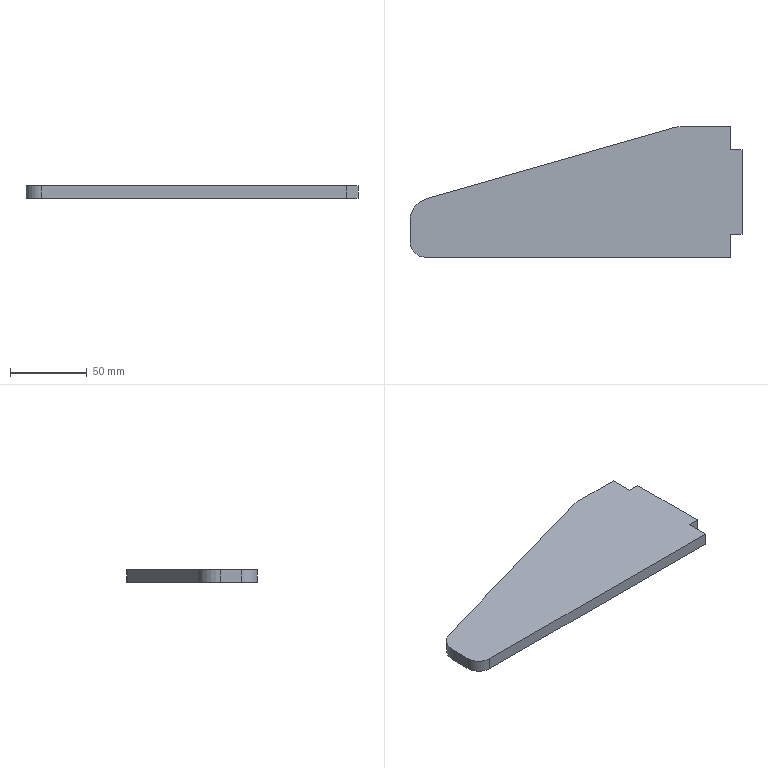Part | SolidWorks | features FlatPattern 1, SMBaseFlange 1, SheetMetal 1 | 1 solid | 14 faces | box 216.5 x 85 x 8 mm | volume 110253 mm3 | plane 11 | cylinder 3 | commonest cylinder face diameters 30 x2 20 x1
STEP:
#1=CARTESIAN_POINT('',(-990.506,559.062,0.));
#2=VERTEX_POINT('',#1);
#3=CARTESIAN_POINT('',(-990.506,574.062,0.));
#4=VERTEX_POINT('',#3);
#5=CARTESIAN_POINT('',(-990.506,559.062,0.));
#6=DIRECTION('',(0.,1.,0.));
#7=VECTOR('',#6,1000.);
#8=LINE('',#5,#7);
#9=EDGE_CURVE('',#2,#4,#8,.T.);
#10=ORIENTED_EDGE('',*,*,#9,.F.);
#11=CARTESIAN_POINT('',(-990.506,559.062,-8.));
#12=VERTEX_POINT('',#11);
#13=CARTESIAN_POINT('',(-990.506,559.062,-8.));
#14=DIRECTION('',(0.,0.,1.));
#15=VECTOR('',#14,1000.);
#16=LINE('',#13,#15);
#17=EDGE_CURVE('',#12,#2,#16,.T.);
#18=ORIENTED_EDGE('',*,*,#17,.F.);
#19=CARTESIAN_POINT('',(-990.506,574.062,-8.));
#20=VERTEX_POINT('',#19);
#21=CARTESIAN_POINT('',(-990.506,559.062,-8.));
#22=DIRECTION('',(0.,1.,0.));
#23=VECTOR('',#22,1000.);
#24=LINE('',#21,#23);
#25=EDGE_CURVE('',#12,#20,#24,.T.);
#26=ORIENTED_EDGE('',*,*,#25,.T.);
#27=CARTESIAN_POINT('',(-990.506,574.062,-8.));
#28=DIRECTION('',(0.,0.,1.));
#29=VECTOR('',#28,1000.);
#30=LINE('',#27,#29);
#31=EDGE_CURVE('',#20,#4,#30,.T.);
#32=ORIENTED_EDGE('',*,*,#31,.T.);
#33=EDGE_LOOP('',(#10,#18,#26,#32));
#34=FACE_OUTER_BOUND('',#33,.T.);
#35=CARTESIAN_POINT('',(-990.506,559.062,-8.));
#36=DIRECTION('',(1.,0.,0.));
#37=DIRECTION('',(0.,0.,-1.));
#38=AXIS2_PLACEMENT_3D('',#35,#36,#37);
#39=PLANE('',#38);
#40=ADVANCED_FACE('',(#34),#39,.T.);
#41=CARTESIAN_POINT('',(-1189.506,559.062,0.));
#42=VERTEX_POINT('',#41);
#43=CARTESIAN_POINT('',(-1189.506,559.062,0.));
#44=DIRECTION('',(1.,0.,0.));
#45=VECTOR('',#44,1000.);
#46=LINE('',#43,#45);
#47=EDGE_CURVE('',#42,#2,#46,.T.);
#48=ORIENTED_EDGE('',*,*,#47,.F.);
#49=CARTESIAN_POINT('',(-1189.506,559.062,-8.));
#50=VERTEX_POINT('',#49);
#51=CARTESIAN_POINT('',(-1189.506,559.062,-8.));
#52=DIRECTION('',(0.,0.,1.));
#53=VECTOR('',#52,1000.);
#54=LINE('',#51,#53);
#55=EDGE_CURVE('',#50,#42,#54,.T.);
#56=ORIENTED_EDGE('',*,*,#55,.F.);
#57=CARTESIAN_POINT('',(-1189.506,559.062,-8.));
#58=DIRECTION('',(1.,0.,0.));
#59=VECTOR('',#58,1000.);
#60=LINE('',#57,#59);
#61=EDGE_CURVE('',#50,#12,#60,.T.);
#62=ORIENTED_EDGE('',*,*,#61,.T.);
#63=ORIENTED_EDGE('',*,*,#17,.T.);
#64=EDGE_LOOP('',(#48,#56,#62,#63));
#65=FACE_OUTER_BOUND('',#64,.T.);
#66=CARTESIAN_POINT('',(-1189.506,559.062,-8.));
#67=DIRECTION('',(0.,-1.,0.));
#68=DIRECTION('',(1.,0.,0.));
#69=AXIS2_PLACEMENT_3D('',#66,#67,#68);
#70=PLANE('',#69);
#71=ADVANCED_FACE('',(#65),#70,.T.);
#72=CARTESIAN_POINT('',(-1199.506,569.062,0.));
#73=VERTEX_POINT('',#72);
#74=CARTESIAN_POINT('',(-1189.506,569.062,0.));
#75=DIRECTION('',(0.,0.,1.));
#76=DIRECTION('',(-1.,0.,0.));
#77=AXIS2_PLACEMENT_3D('',#74,#75,#76);
#78=CIRCLE('',#77,10.);
#79=EDGE_CURVE('',#73,#42,#78,.T.);
#80=ORIENTED_EDGE('',*,*,#79,.F.);
#81=CARTESIAN_POINT('',(-1199.506,569.062,-8.));
#82=VERTEX_POINT('',#81);
#83=CARTESIAN_POINT('',(-1199.506,569.062,-8.));
#84=DIRECTION('',(0.,0.,1.));
#85=VECTOR('',#84,1000.);
#86=LINE('',#83,#85);
#87=EDGE_CURVE('',#82,#73,#86,.T.);
#88=ORIENTED_EDGE('',*,*,#87,.F.);
#89=CARTESIAN_POINT('',(-1189.506,569.062,-8.));
#90=DIRECTION('',(0.,0.,1.));
#91=DIRECTION('',(-1.,0.,0.));
#92=AXIS2_PLACEMENT_3D('',#89,#90,#91);
#93=CIRCLE('',#92,10.);
#94=EDGE_CURVE('',#82,#50,#93,.T.);
#95=ORIENTED_EDGE('',*,*,#94,.T.);
#96=ORIENTED_EDGE('',*,*,#55,.T.);
#97=EDGE_LOOP('',(#80,#88,#95,#96));
#98=FACE_OUTER_BOUND('',#97,.T.);
#99=CARTESIAN_POINT('',(-1189.506,569.062,-8.));
#100=DIRECTION('',(0.,0.,1.));
#101=DIRECTION('',(1.,0.,0.));
#102=AXIS2_PLACEMENT_3D('',#99,#100,#101);
#103=CYLINDRICAL_SURFACE('',#102,10.);
#104=ADVANCED_FACE('',(#98),#103,.T.);
#105=CARTESIAN_POINT('',(-1199.506,582.765,0.));
#106=VERTEX_POINT('',#105);
#107=CARTESIAN_POINT('',(-1199.506,582.765,0.));
#108=DIRECTION('',(0.,-1.,0.));
#109=VECTOR('',#108,1000.);
#110=LINE('',#107,#109);
#111=EDGE_CURVE('',#106,#73,#110,.T.);
#112=ORIENTED_EDGE('',*,*,#111,.F.);
#113=CARTESIAN_POINT('',(-1199.506,582.765,-8.));
#114=VERTEX_POINT('',#113);
#115=CARTESIAN_POINT('',(-1199.506,582.765,-8.));
#116=DIRECTION('',(0.,0.,1.));
#117=VECTOR('',#116,1000.);
#118=LINE('',#115,#117);
#119=EDGE_CURVE('',#114,#106,#118,.T.);
#120=ORIENTED_EDGE('',*,*,#119,.F.);
#121=CARTESIAN_POINT('',(-1199.506,582.765,-8.));
#122=DIRECTION('',(0.,-1.,0.));
#123=VECTOR('',#122,1000.);
#124=LINE('',#121,#123);
#125=EDGE_CURVE('',#114,#82,#124,.T.);
#126=ORIENTED_EDGE('',*,*,#125,.T.);
#127=ORIENTED_EDGE('',*,*,#87,.T.);
#128=EDGE_LOOP('',(#112,#120,#126,#127));
#129=FACE_OUTER_BOUND('',#128,.T.);
#130=CARTESIAN_POINT('',(-1199.506,582.765,-8.));
#131=DIRECTION('',(-1.,0.,0.));
#132=DIRECTION('',(0.,0.,1.));
#133=AXIS2_PLACEMENT_3D('',#130,#131,#132);
#134=PLANE('',#133);
#135=ADVANCED_FACE('',(#129),#134,.T.);
#136=CARTESIAN_POINT('',(-1188.648,597.182,0.));
#137=VERTEX_POINT('',#136);
#138=CARTESIAN_POINT('',(-1184.506,582.765,0.));
#139=DIRECTION('',(0.,0.,1.));
#140=DIRECTION('',(1.,0.,0.));
#141=AXIS2_PLACEMENT_3D('',#138,#139,#140);
#142=CIRCLE('',#141,15.);
#143=EDGE_CURVE('',#137,#106,#142,.T.);
#144=ORIENTED_EDGE('',*,*,#143,.F.);
#145=CARTESIAN_POINT('',(-1188.648,597.182,-8.));
#146=VERTEX_POINT('',#145);
#147=CARTESIAN_POINT('',(-1188.648,597.182,-8.));
#148=DIRECTION('',(0.,0.,1.));
#149=VECTOR('',#148,1000.);
#150=LINE('',#147,#149);
#151=EDGE_CURVE('',#146,#137,#150,.T.);
#152=ORIENTED_EDGE('',*,*,#151,.F.);
#153=CARTESIAN_POINT('',(-1184.506,582.765,-8.));
#154=DIRECTION('',(0.,0.,1.));
#155=DIRECTION('',(1.,0.,0.));
#156=AXIS2_PLACEMENT_3D('',#153,#154,#155);
#157=CIRCLE('',#156,15.);
#158=EDGE_CURVE('',#146,#114,#157,.T.);
#159=ORIENTED_EDGE('',*,*,#158,.T.);
#160=ORIENTED_EDGE('',*,*,#119,.T.);
#161=EDGE_LOOP('',(#144,#152,#159,#160));
#162=FACE_OUTER_BOUND('',#161,.T.);
#163=CARTESIAN_POINT('',(-1184.506,582.765,-8.));
#164=DIRECTION('',(0.,0.,1.));
#165=DIRECTION('',(1.,0.,0.));
#166=AXIS2_PLACEMENT_3D('',#163,#164,#165);
#167=CYLINDRICAL_SURFACE('',#166,15.);
#168=ADVANCED_FACE('',(#162),#167,.T.);
#169=CARTESIAN_POINT('',(-1027.536,643.478,0.));
#170=VERTEX_POINT('',#169);
#171=CARTESIAN_POINT('',(-1027.536,643.478,0.));
#172=DIRECTION('',(-0.9611,-0.2762,0.));
#173=VECTOR('',#172,1000.);
#174=LINE('',#171,#173);
#175=EDGE_CURVE('',#170,#137,#174,.T.);
#176=ORIENTED_EDGE('',*,*,#175,.F.);
#177=CARTESIAN_POINT('',(-1027.536,643.478,-8.));
#178=VERTEX_POINT('',#177);
#179=CARTESIAN_POINT('',(-1027.536,643.478,-8.));
#180=DIRECTION('',(0.,0.,1.));
#181=VECTOR('',#180,1000.);
#182=LINE('',#179,#181);
#183=EDGE_CURVE('',#178,#170,#182,.T.);
#184=ORIENTED_EDGE('',*,*,#183,.F.);
#185=CARTESIAN_POINT('',(-1027.536,643.478,-8.));
#186=DIRECTION('',(-0.9611,-0.2762,0.));
#187=VECTOR('',#186,1000.);
#188=LINE('',#185,#187);
#189=EDGE_CURVE('',#178,#146,#188,.T.);
#190=ORIENTED_EDGE('',*,*,#189,.T.);
#191=ORIENTED_EDGE('',*,*,#151,.T.);
#192=EDGE_LOOP('',(#176,#184,#190,#191));
#193=FACE_OUTER_BOUND('',#192,.T.);
#194=CARTESIAN_POINT('',(-1027.536,643.478,-8.));
#195=DIRECTION('',(-0.2762,0.9611,0.));
#196=DIRECTION('',(-0.9611,-0.2762,0.));
#197=AXIS2_PLACEMENT_3D('',#194,#195,#196);
#198=PLANE('',#197);
#199=ADVANCED_FACE('',(#193),#198,.T.);
#200=CARTESIAN_POINT('',(-1023.393,644.062,0.));
#201=VERTEX_POINT('',#200);
#202=CARTESIAN_POINT('',(-1023.393,629.062,0.));
#203=DIRECTION('',(0.,0.,1.));
#204=DIRECTION('',(1.,0.,0.));
#205=AXIS2_PLACEMENT_3D('',#202,#203,#204);
#206=CIRCLE('',#205,15.);
#207=EDGE_CURVE('',#201,#170,#206,.T.);
#208=ORIENTED_EDGE('',*,*,#207,.F.);
#209=CARTESIAN_POINT('',(-1023.393,644.062,-8.));
#210=VERTEX_POINT('',#209);
#211=CARTESIAN_POINT('',(-1023.393,644.062,-8.));
#212=DIRECTION('',(0.,0.,1.));
#213=VECTOR('',#212,1000.);
#214=LINE('',#211,#213);
#215=EDGE_CURVE('',#210,#201,#214,.T.);
#216=ORIENTED_EDGE('',*,*,#215,.F.);
#217=CARTESIAN_POINT('',(-1023.393,629.062,-8.));
#218=DIRECTION('',(0.,0.,1.));
#219=DIRECTION('',(1.,0.,0.));
#220=AXIS2_PLACEMENT_3D('',#217,#218,#219);
#221=CIRCLE('',#220,15.);
#222=EDGE_CURVE('',#210,#178,#221,.T.);
#223=ORIENTED_EDGE('',*,*,#222,.T.);
#224=ORIENTED_EDGE('',*,*,#183,.T.);
#225=EDGE_LOOP('',(#208,#216,#223,#224));
#226=FACE_OUTER_BOUND('',#225,.T.);
#227=CARTESIAN_POINT('',(-1023.393,629.062,-8.));
#228=DIRECTION('',(0.,0.,1.));
#229=DIRECTION('',(1.,0.,0.));
#230=AXIS2_PLACEMENT_3D('',#227,#228,#229);
#231=CYLINDRICAL_SURFACE('',#230,15.);
#232=ADVANCED_FACE('',(#226),#231,.T.);
#233=CARTESIAN_POINT('',(-990.506,644.062,0.));
#234=VERTEX_POINT('',#233);
#235=CARTESIAN_POINT('',(-990.506,644.062,0.));
#236=DIRECTION('',(-1.,0.,0.));
#237=VECTOR('',#236,1000.);
#238=LINE('',#235,#237);
#239=EDGE_CURVE('',#234,#201,#238,.T.);
#240=ORIENTED_EDGE('',*,*,#239,.F.);
#241=CARTESIAN_POINT('',(-990.506,644.062,-8.));
#242=VERTEX_POINT('',#241);
#243=CARTESIAN_POINT('',(-990.506,644.062,-8.));
#244=DIRECTION('',(0.,0.,1.));
#245=VECTOR('',#244,1000.);
#246=LINE('',#243,#245);
#247=EDGE_CURVE('',#242,#234,#246,.T.);
#248=ORIENTED_EDGE('',*,*,#247,.F.);
#249=CARTESIAN_POINT('',(-990.506,644.062,-8.));
#250=DIRECTION('',(-1.,0.,0.));
#251=VECTOR('',#250,1000.);
#252=LINE('',#249,#251);
#253=EDGE_CURVE('',#242,#210,#252,.T.);
#254=ORIENTED_EDGE('',*,*,#253,.T.);
#255=ORIENTED_EDGE('',*,*,#215,.T.);
#256=EDGE_LOOP('',(#240,#248,#254,#255));
#257=FACE_OUTER_BOUND('',#256,.T.);
#258=CARTESIAN_POINT('',(-990.506,644.062,-8.));
#259=DIRECTION('',(0.,1.,0.));
#260=DIRECTION('',(0.,0.,1.));
#261=AXIS2_PLACEMENT_3D('',#258,#259,#260);
#262=PLANE('',#261);
#263=ADVANCED_FACE('',(#257),#262,.T.);
#264=CARTESIAN_POINT('',(-990.506,629.062,0.));
#265=VERTEX_POINT('',#264);
#266=CARTESIAN_POINT('',(-990.506,629.062,0.));
#267=DIRECTION('',(0.,1.,0.));
#268=VECTOR('',#267,1000.);
#269=LINE('',#266,#268);
#270=EDGE_CURVE('',#265,#234,#269,.T.);
#271=ORIENTED_EDGE('',*,*,#270,.F.);
#272=CARTESIAN_POINT('',(-990.506,629.062,-8.));
#273=VERTEX_POINT('',#272);
#274=CARTESIAN_POINT('',(-990.506,629.062,-8.));
#275=DIRECTION('',(0.,0.,1.));
#276=VECTOR('',#275,1000.);
#277=LINE('',#274,#276);
#278=EDGE_CURVE('',#273,#265,#277,.T.);
#279=ORIENTED_EDGE('',*,*,#278,.F.);
#280=CARTESIAN_POINT('',(-990.506,629.062,-8.));
#281=DIRECTION('',(0.,1.,0.));
#282=VECTOR('',#281,1000.);
#283=LINE('',#280,#282);
#284=EDGE_CURVE('',#273,#242,#283,.T.);
#285=ORIENTED_EDGE('',*,*,#284,.T.);
#286=ORIENTED_EDGE('',*,*,#247,.T.);
#287=EDGE_LOOP('',(#271,#279,#285,#286));
#288=FACE_OUTER_BOUND('',#287,.T.);
#289=CARTESIAN_POINT('',(-990.506,629.062,-8.));
#290=DIRECTION('',(1.,0.,0.));
#291=DIRECTION('',(0.,0.,-1.));
#292=AXIS2_PLACEMENT_3D('',#289,#290,#291);
#293=PLANE('',#292);
#294=ADVANCED_FACE('',(#288),#293,.T.);
#295=CARTESIAN_POINT('',(-983.006,629.062,0.));
#296=VERTEX_POINT('',#295);
#297=CARTESIAN_POINT('',(-983.006,629.062,0.));
#298=DIRECTION('',(-1.,0.,0.));
#299=VECTOR('',#298,1000.);
#300=LINE('',#297,#299);
#301=EDGE_CURVE('',#296,#265,#300,.T.);
#302=ORIENTED_EDGE('',*,*,#301,.F.);
#303=CARTESIAN_POINT('',(-983.006,629.062,-8.));
#304=VERTEX_POINT('',#303);
#305=CARTESIAN_POINT('',(-983.006,629.062,-8.));
#306=DIRECTION('',(0.,0.,1.));
#307=VECTOR('',#306,1000.);
#308=LINE('',#305,#307);
#309=EDGE_CURVE('',#304,#296,#308,.T.);
#310=ORIENTED_EDGE('',*,*,#309,.F.);
#311=CARTESIAN_POINT('',(-983.006,629.062,-8.));
#312=DIRECTION('',(-1.,0.,0.));
#313=VECTOR('',#312,1000.);
#314=LINE('',#311,#313);
#315=EDGE_CURVE('',#304,#273,#314,.T.);
#316=ORIENTED_EDGE('',*,*,#315,.T.);
#317=ORIENTED_EDGE('',*,*,#278,.T.);
#318=EDGE_LOOP('',(#302,#310,#316,#317));
#319=FACE_OUTER_BOUND('',#318,.T.);
#320=CARTESIAN_POINT('',(-983.006,629.062,-8.));
#321=DIRECTION('',(0.,1.,0.));
#322=DIRECTION('',(0.,0.,1.));
#323=AXIS2_PLACEMENT_3D('',#320,#321,#322);
#324=PLANE('',#323);
#325=ADVANCED_FACE('',(#319),#324,.T.);
#326=CARTESIAN_POINT('',(-983.006,574.062,0.));
#327=VERTEX_POINT('',#326);
#328=CARTESIAN_POINT('',(-983.006,574.062,0.));
#329=DIRECTION('',(0.,1.,0.));
#330=VECTOR('',#329,1000.);
#331=LINE('',#328,#330);
#332=EDGE_CURVE('',#327,#296,#331,.T.);
#333=ORIENTED_EDGE('',*,*,#332,.F.);
#334=CARTESIAN_POINT('',(-983.006,574.062,-8.));
#335=VERTEX_POINT('',#334);
#336=CARTESIAN_POINT('',(-983.006,574.062,-8.));
#337=DIRECTION('',(0.,0.,1.));
#338=VECTOR('',#337,1000.);
#339=LINE('',#336,#338);
#340=EDGE_CURVE('',#335,#327,#339,.T.);
#341=ORIENTED_EDGE('',*,*,#340,.F.);
#342=CARTESIAN_POINT('',(-983.006,574.062,-8.));
#343=DIRECTION('',(0.,1.,0.));
#344=VECTOR('',#343,1000.);
#345=LINE('',#342,#344);
#346=EDGE_CURVE('',#335,#304,#345,.T.);
#347=ORIENTED_EDGE('',*,*,#346,.T.);
#348=ORIENTED_EDGE('',*,*,#309,.T.);
#349=EDGE_LOOP('',(#333,#341,#347,#348));
#350=FACE_OUTER_BOUND('',#349,.T.);
#351=CARTESIAN_POINT('',(-983.006,574.062,-8.));
#352=DIRECTION('',(1.,0.,0.));
#353=DIRECTION('',(0.,0.,-1.));
#354=AXIS2_PLACEMENT_3D('',#351,#352,#353);
#355=PLANE('',#354);
#356=ADVANCED_FACE('',(#350),#355,.T.);
#357=CARTESIAN_POINT('',(-990.506,574.062,0.));
#358=DIRECTION('',(1.,0.,0.));
#359=VECTOR('',#358,1000.);
#360=LINE('',#357,#359);
#361=EDGE_CURVE('',#4,#327,#360,.T.);
#362=ORIENTED_EDGE('',*,*,#361,.F.);
#363=ORIENTED_EDGE('',*,*,#31,.F.);
#364=CARTESIAN_POINT('',(-990.506,574.062,-8.));
#365=DIRECTION('',(1.,0.,0.));
#366=VECTOR('',#365,1000.);
#367=LINE('',#364,#366);
#368=EDGE_CURVE('',#20,#335,#367,.T.);
#369=ORIENTED_EDGE('',*,*,#368,.T.);
#370=ORIENTED_EDGE('',*,*,#340,.T.);
#371=EDGE_LOOP('',(#362,#363,#369,#370));
#372=FACE_OUTER_BOUND('',#371,.T.);
#373=CARTESIAN_POINT('',(-990.506,574.062,-8.));
#374=DIRECTION('',(0.,-1.,0.));
#375=DIRECTION('',(0.,0.,-1.));
#376=AXIS2_PLACEMENT_3D('',#373,#374,#375);
#377=PLANE('',#376);
#378=ADVANCED_FACE('',(#372),#377,.T.);
#379=ORIENTED_EDGE('',*,*,#25,.F.);
#380=ORIENTED_EDGE('',*,*,#61,.F.);
#381=ORIENTED_EDGE('',*,*,#94,.F.);
#382=ORIENTED_EDGE('',*,*,#125,.F.);
#383=ORIENTED_EDGE('',*,*,#158,.F.);
#384=ORIENTED_EDGE('',*,*,#189,.F.);
#385=ORIENTED_EDGE('',*,*,#222,.F.);
#386=ORIENTED_EDGE('',*,*,#253,.F.);
#387=ORIENTED_EDGE('',*,*,#284,.F.);
#388=ORIENTED_EDGE('',*,*,#315,.F.);
#389=ORIENTED_EDGE('',*,*,#346,.F.);
#390=ORIENTED_EDGE('',*,*,#368,.F.);
#391=EDGE_LOOP('',(#379,#380,#381,#382,#383,#384,#385,#386,#387,#388,#389,#390));
#392=FACE_OUTER_BOUND('',#391,.T.);
#393=CARTESIAN_POINT('',(-1023.393,629.062,-8.));
#394=DIRECTION('',(0.,0.,1.));
#395=DIRECTION('',(1.,0.,0.));
#396=AXIS2_PLACEMENT_3D('',#393,#394,#395);
#397=PLANE('',#396);
#398=ADVANCED_FACE('',(#392),#397,.F.);
#399=ORIENTED_EDGE('',*,*,#9,.T.);
#400=ORIENTED_EDGE('',*,*,#361,.T.);
#401=ORIENTED_EDGE('',*,*,#332,.T.);
#402=ORIENTED_EDGE('',*,*,#301,.T.);
#403=ORIENTED_EDGE('',*,*,#270,.T.);
#404=ORIENTED_EDGE('',*,*,#239,.T.);
#405=ORIENTED_EDGE('',*,*,#207,.T.);
#406=ORIENTED_EDGE('',*,*,#175,.T.);
#407=ORIENTED_EDGE('',*,*,#143,.T.);
#408=ORIENTED_EDGE('',*,*,#111,.T.);
#409=ORIENTED_EDGE('',*,*,#79,.T.);
#410=ORIENTED_EDGE('',*,*,#47,.T.);
#411=EDGE_LOOP('',(#399,#400,#401,#402,#403,#404,#405,#406,#407,#408,#409,#410));
#412=FACE_OUTER_BOUND('',#411,.T.);
#413=CARTESIAN_POINT('',(-1023.393,629.062,0.));
#414=DIRECTION('',(0.,0.,1.));
#415=DIRECTION('',(1.,0.,0.));
#416=AXIS2_PLACEMENT_3D('',#413,#414,#415);
#417=PLANE('',#416);
#418=ADVANCED_FACE('',(#412),#417,.T.);
#419=CLOSED_SHELL('',(#40,#71,#104,#135,#168,#199,#232,#263,#294,#325,#356,#378,#398,#418));
#420=MANIFOLD_SOLID_BREP('',#419);
#421=CARTESIAN_POINT('',(0.,0.,0.));
#422=DIRECTION('',(0.,0.,1.));
#423=DIRECTION('',(1.,0.,0.));
#424=AXIS2_PLACEMENT_3D('',#421,#422,#423);
#425=(LENGTH_UNIT()NAMED_UNIT(*)SI_UNIT(.MILLI.,.METRE.));
#426=UNCERTAINTY_MEASURE_WITH_UNIT(LENGTH_MEASURE(0.00001),#425,'','');
#427=(NAMED_UNIT(*)PLANE_ANGLE_UNIT()SI_UNIT($,.RADIAN.));
#428=(NAMED_UNIT(*)SI_UNIT($,.STERADIAN.)SOLID_ANGLE_UNIT());
#429=(GEOMETRIC_REPRESENTATION_CONTEXT(3)GLOBAL_UNCERTAINTY_ASSIGNED_CONTEXT((#426))GLOBAL_UNIT_ASSIGNED_CONTEXT((#425,#427,#428))REPRESENTATION_CONTEXT('',''));
#430=ADVANCED_BREP_SHAPE_REPRESENTATION('',(#420,#424),#429);